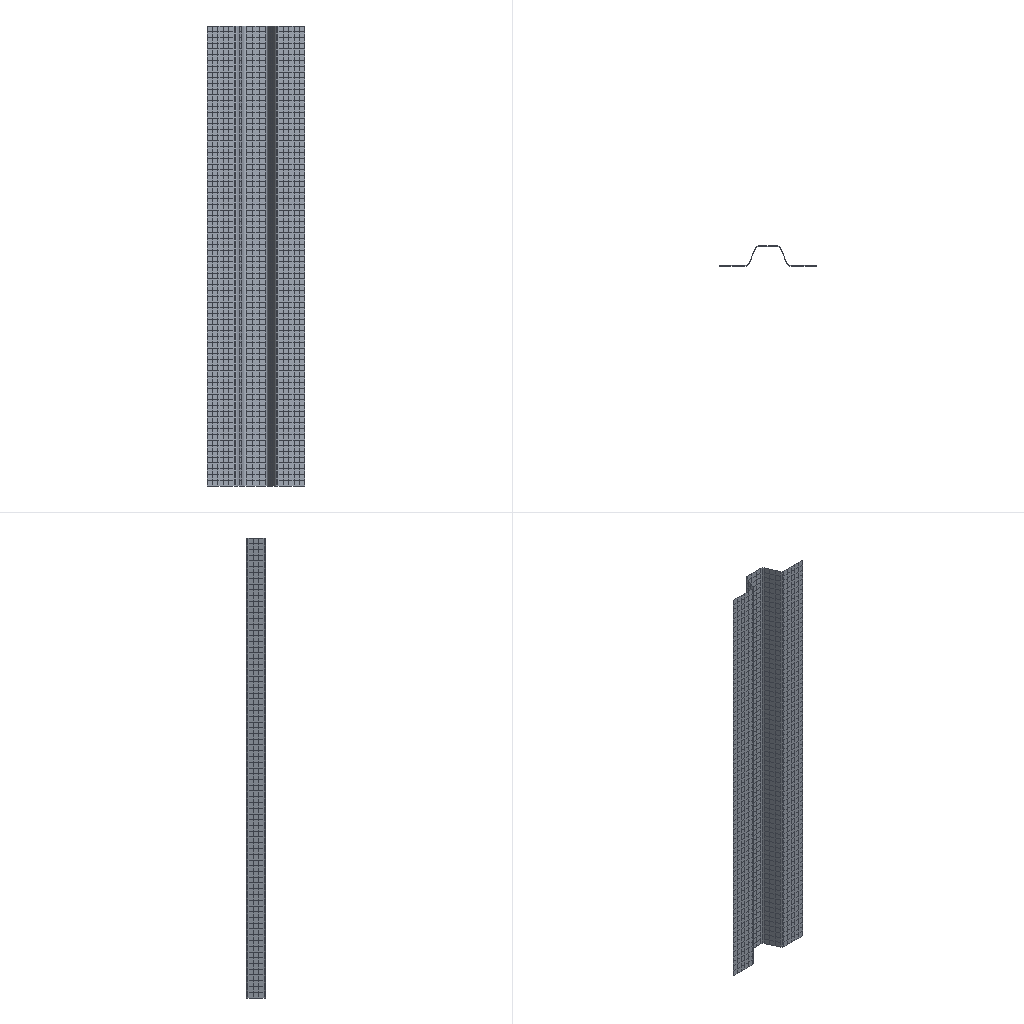Simulation study | abaqus
Set-up summary:
category,name,step,type,value,unit,region
solver,abaqus
solver,version,,,Abaqus/Standard 2020
units,not stated in the deck,,not stated
analysis,deck,,static,static
load_step,Step-1,Step-1,static
load_step,requested,,,1
mesh,nodes,,,4536
mesh,elements,,,4320
element_type,S4R,,shell,4320
load,load commands in deck,,count,1
bc,support commands in deck,,count,1
material,MATERIAL-1,,in results
check,setup vs results,,match,"per instance, exact: element labels, types and connectivity; labels of the nodes the elements use; coordinates of those nodes at SINGLE_PRECISION in 2 of 2 instance(s)"
Abaqus input file, long lists of numbers shortened:
*Heading
** Job name: Job-1 Model name: Model-1
** Generated by: Abaqus/CAE 2020
*Preprint, echo=NO, model=NO, history=NO, contact=NO
**
** PARTS
**
*Part, name=Part-1
*Node
      1,  -33.685,   2.982,         800.
      2,  -38.259,           0.,         800.
** (2266 more lines like these left out)
*Element, type=S4R
  1,   1,  21, 847, 180
  2,  21,   2,  22, 847
** (2158 more lines like these left out)
*Nset, nset=Set-1, generate
    1,  2268,     1
*Elset, elset=Set-1, generate
    1,  2160,     1
** Region: (CompositeLayup-1-1: Generated From Layup)
*Elset, elset=CompositeLayup-1-1, generate
    1,  2160,     1
** Section: CompositeLayup-1-1
*Shell Section, elset=CompositeLayup-1-1, composite, layup=CompositeLayup-1
1., 3, Material-1, 0., 层-1
1., 3, Material-1, 45., 层-2
1., 3, Material-1, 0., 层-3
1., 3, Material-1, -45., 层-4
1., 3, Material-1, 90., 层-5
1., 3, Material-1, 45., 层-6
1., 3, Material-1, 0., 层-7
1., 3, Material-1, -45., 层-8
1., 3, Material-1, 90., 层-9
1., 3, Material-1, 90., 层-10
1., 3, Material-1, -45., 层-11
1., 3, Material-1, 0., 层-12
1., 3, Material-1, 45., 层-13
1., 3, Material-1, 90., 层-14
1., 3, Material-1, -45., 层-15
1., 3, Material-1, 0., 层-16
1., 3, Material-1, 45., 层-17
1., 3, Material-1, 0., 层-18
*End Part
**
**
** ASSEMBLY
**
*Assembly, name=Assembly
**
*Instance, name=Part-1-1, part=Part-1
*End Instance
**
*Instance, name=Part-1-2, part=Part-1
*End Instance
**
*Nset, nset=Set-1, instance=Part-1-1, generate
    1,  2268,     1
*Nset, nset=Set-1, instance=Part-1-2, generate
    1,  2268,     1
*Elset, elset=Set-1, instance=Part-1-1, generate
    1,  2160,     1
*Elset, elset=Set-1, instance=Part-1-2, generate
    1,  2160,     1
*Nset, nset=Set-2, instance=Part-1-1, generate
    1,  2268,     1
*Nset, nset=Set-2, instance=Part-1-2, generate
    1,  2268,     1
*Elset, elset=Set-2, instance=Part-1-1, generate
    1,  2160,     1
*Elset, elset=Set-2, instance=Part-1-2, generate
    1,  2160,     1
*Nset, nset=Set-3, instance=Part-1-2
  19,  20, 762, 763, 764, 765, 766, 767, 768, 769, 770, 771, 772, 773, 774, 775
 776, 777, 778, 779, 780, 781, 782, 783, 784, 785, 786, 787, 788, 789, 790, 791
** (4 more lines like these left out)
*Elset, elset=Set-3, instance=Part-1-2, generate
 1921,  2000,     1
*Nset, nset=Set-4, instance=Part-1-2
   1,   2,   6,   7,   9,  12,  13,  14,  17,  20,  21, 262, 263, 264, 265, 266
 267, 351, 513, 514, 515, 675, 676, 841, 842, 843, 844, 845
*Elset, elset=Set-4, instance=Part-1-2
    1,    2,  161,  241,  321,  480,  560,  640,  720,  800,  801,  802,  961, 1041, 1121, 1201
 1202, 1440, 1520, 1600, 1601, 1681, 1761, 1841, 1921, 2001, 2002
*End Assembly
**
** MATERIALS
**
*Material, name=Material-1
*Conductivity
500.,
*Density
 1.5e-09,
*Elastic, type=ENGINEERING CONSTANTS
181000.,10300.,10300.,  0.28,  0.28,  0.28, 7170., 7170.
 3585.,
*Expansion, type=ANISO
 2e-08, 2.25e-05, 2.25e-05,       0.,       0.,       0.
*Specific Heat
 4.6e+08,
**
** PHYSICAL CONSTANTS
**
*Physical Constants, absolute zero=-273., stefan boltzmann=5.67e-08
**
** PREDEFINED FIELDS
**
** Name: Predefined Field-1   Type: Temperature
*Initial Conditions, type=TEMPERATURE
Set-1, 180.
** ----------------------------------------------------------------
**
** STEP: Step-1
**
*Step, name=Step-1, nlgeom=YES, inc=1000
*Static, stabilize=0.0002, allsdtol=0.05, continue=NO
0.001, 1., 1e-05, 1.
**
** BOUNDARY CONDITIONS
**
** Name: BC-1 Type: 对称/反对称/完全固定
*Boundary
Set-4, ENCASTRE
**
** PREDEFINED FIELDS
**
** Name: Predefined Field-2   Type: Temperature
*Temperature
Set-2, 20.
**
** OUTPUT REQUESTS
**
*Restart, write, frequency=0
**
** FIELD OUTPUT: F-Output-1
**
*Output, field
*Node Output
CF, NT, RF, U, V
*Element Output, directions=YES
E, LE, MISES, PE, PEEQ, PEMAG, S, TEMP
*Contact Output
CDISP, CSTRESS
**
** HISTORY OUTPUT: H-Output-1
**
*Output, history, variable=PRESELECT
*End Step
Results summary:
result,step,,completed,increments=17 time=1.0/1.0
result,analysis,,,static
result,last_loadstep,,,1
result,primary field,,,"U, UR"
result,reaction total,,FX,0.07326,model units
result,reaction total,,FY,-2.847,model units
result,reaction total,,FZ,51.554,model units